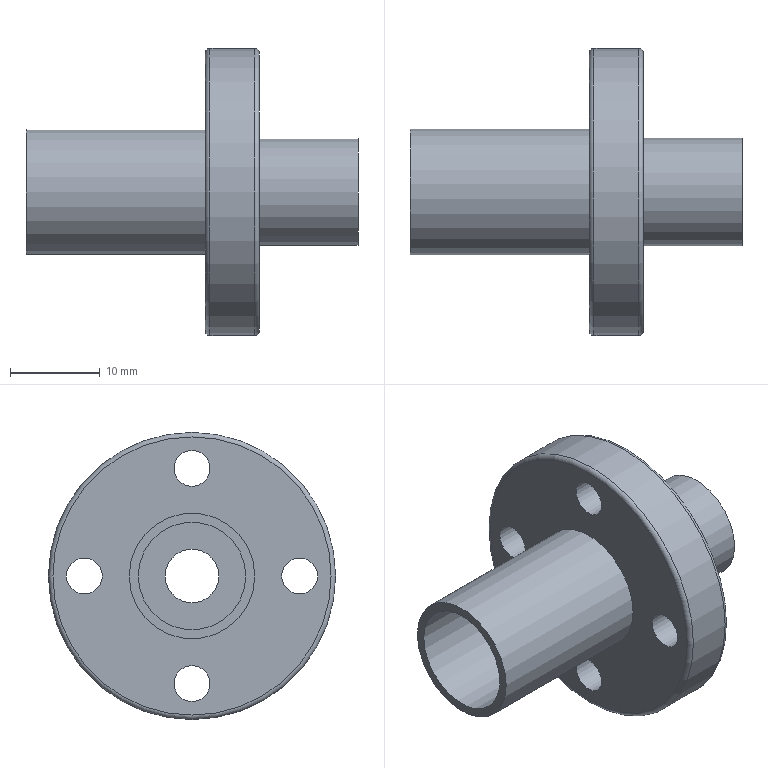Part | STEP file | 1-23.1 | 1 solid | 16 faces | box 37 x 32 x 32 mm | volume 6942 mm3 | cylinder 9 | plane 5 | torus 2 | commonest cylinder face diameters 4 x4 12 x2 6 x1 14 x1 32 x1
STEP:
#1=CARTESIAN_POINT('',(0.,0.,0.));
#2=DIRECTION('',(0.,0.,1.));
#3=DIRECTION('',(1.,0.,0.));
#4=AXIS2_PLACEMENT_3D('',#1,#2,#3);
#5=CARTESIAN_POINT('',(0.,2.,12.));
#6=VERTEX_POINT('',#5);
#7=CARTESIAN_POINT('',(6.,2.,12.));
#8=VERTEX_POINT('',#7);
#9=CARTESIAN_POINT('',(0.,2.,12.));
#10=DIRECTION('',(1.,0.,0.));
#11=VECTOR('',#10,1.);
#12=LINE('',#9,#11);
#13=CARTESIAN_POINT('',(0.,0.,12.));
#14=DIRECTION('',(1.,0.,0.));
#15=DIRECTION('',(0.,1.,0.));
#16=AXIS2_PLACEMENT_3D('',#13,#14,#15);
#17=CYLINDRICAL_SURFACE('',#16,2.);
#18=CARTESIAN_POINT('',(6.283,0.));
#19=DIRECTION('',(0.,1.));
#20=VECTOR('',#19,1.);
#21=LINE('',#18,#20);
#22=(GEOMETRIC_REPRESENTATION_CONTEXT(2)PARAMETRIC_REPRESENTATION_CONTEXT()REPRESENTATION_CONTEXT('',''));
#23=DEFINITIONAL_REPRESENTATION('',(#21),#22);
#24=PCURVE('',#17,#23);
#25=CARTESIAN_POINT('',(0.,0.));
#26=DIRECTION('',(0.,1.));
#27=VECTOR('',#26,1.);
#28=LINE('',#25,#27);
#29=(GEOMETRIC_REPRESENTATION_CONTEXT(2)PARAMETRIC_REPRESENTATION_CONTEXT()REPRESENTATION_CONTEXT('',''));
#30=DEFINITIONAL_REPRESENTATION('',(#28),#29);
#31=PCURVE('',#17,#30);
#32=SEAM_CURVE('',#12,(#24,#31),.PCURVE_S1.);
#33=EDGE_CURVE('',#6,#8,#32,.T.);
#34=ORIENTED_EDGE('',*,*,#33,.T.);
#35=CARTESIAN_POINT('',(6.,0.,12.));
#36=DIRECTION('',(-1.,0.,0.));
#37=DIRECTION('',(0.,1.,0.));
#38=AXIS2_PLACEMENT_3D('',#35,#36,#37);
#39=CIRCLE('',#38,2.);
#40=CARTESIAN_POINT('',(6.283,6.));
#41=DIRECTION('',(-1.,0.));
#42=VECTOR('',#41,1.);
#43=LINE('',#40,#42);
#44=(GEOMETRIC_REPRESENTATION_CONTEXT(2)PARAMETRIC_REPRESENTATION_CONTEXT()REPRESENTATION_CONTEXT('',''));
#45=DEFINITIONAL_REPRESENTATION('',(#43),#44);
#46=PCURVE('',#17,#45);
#47=CARTESIAN_POINT('',(6.,-4.287,0.));
#48=DIRECTION('',(1.,0.,0.));
#49=DIRECTION('',(0.,1.,0.));
#50=AXIS2_PLACEMENT_3D('',#47,#48,#49);
#51=PLANE('',#50);
#52=CARTESIAN_POINT('',(6.287,12.));
#53=CARTESIAN_POINT('',(6.287,8.536));
#54=CARTESIAN_POINT('',(3.287,10.268));
#55=CARTESIAN_POINT('',(0.2872,12.));
#56=CARTESIAN_POINT('',(3.287,13.732));
#57=CARTESIAN_POINT('',(6.287,15.464));
#58=CARTESIAN_POINT('',(6.287,12.));
#59=(BOUNDED_CURVE()B_SPLINE_CURVE(2,(#52,#53,#54,#55,#56,#57,#58),.UNSPECIFIED.,.T.,.F.)B_SPLINE_CURVE_WITH_KNOTS((1,2,2,2,2,1),(-2.094,0.,2.094,4.189,6.283,8.378),.UNSPECIFIED.)CURVE()GEOMETRIC_REPRESENTATION_ITEM()RATIONAL_B_SPLINE_CURVE((1.,0.5,1.,0.5,1.,0.5,1.))REPRESENTATION_ITEM(''));
#60=(GEOMETRIC_REPRESENTATION_CONTEXT(2)PARAMETRIC_REPRESENTATION_CONTEXT()REPRESENTATION_CONTEXT('',''));
#61=DEFINITIONAL_REPRESENTATION('',(#59),#60);
#62=PCURVE('',#51,#61);
#63=SURFACE_CURVE('',#39,(#46,#62),.PCURVE_S1.);
#64=EDGE_CURVE('',#8,#8,#63,.T.);
#65=ORIENTED_EDGE('',*,*,#64,.T.);
#66=ORIENTED_EDGE('',*,*,#33,.F.);
#67=CARTESIAN_POINT('',(0.,0.,12.));
#68=DIRECTION('',(-1.,0.,0.));
#69=DIRECTION('',(0.,1.,0.));
#70=AXIS2_PLACEMENT_3D('',#67,#68,#69);
#71=CIRCLE('',#70,2.);
#72=CARTESIAN_POINT('',(6.283,0.));
#73=DIRECTION('',(-1.,0.));
#74=VECTOR('',#73,1.);
#75=LINE('',#72,#74);
#76=(GEOMETRIC_REPRESENTATION_CONTEXT(2)PARAMETRIC_REPRESENTATION_CONTEXT()REPRESENTATION_CONTEXT('',''));
#77=DEFINITIONAL_REPRESENTATION('',(#75),#76);
#78=PCURVE('',#17,#77);
#79=CARTESIAN_POINT('',(0.,-4.287,0.));
#80=DIRECTION('',(1.,0.,0.));
#81=DIRECTION('',(0.,1.,0.));
#82=AXIS2_PLACEMENT_3D('',#79,#80,#81);
#83=PLANE('',#82);
#84=CARTESIAN_POINT('',(6.287,12.));
#85=CARTESIAN_POINT('',(6.287,8.536));
#86=CARTESIAN_POINT('',(3.287,10.268));
#87=CARTESIAN_POINT('',(0.2872,12.));
#88=CARTESIAN_POINT('',(3.287,13.732));
#89=CARTESIAN_POINT('',(6.287,15.464));
#90=CARTESIAN_POINT('',(6.287,12.));
#91=(BOUNDED_CURVE()B_SPLINE_CURVE(2,(#84,#85,#86,#87,#88,#89,#90),.UNSPECIFIED.,.T.,.F.)B_SPLINE_CURVE_WITH_KNOTS((1,2,2,2,2,1),(-2.094,0.,2.094,4.189,6.283,8.378),.UNSPECIFIED.)CURVE()GEOMETRIC_REPRESENTATION_ITEM()RATIONAL_B_SPLINE_CURVE((1.,0.5,1.,0.5,1.,0.5,1.))REPRESENTATION_ITEM(''));
#92=(GEOMETRIC_REPRESENTATION_CONTEXT(2)PARAMETRIC_REPRESENTATION_CONTEXT()REPRESENTATION_CONTEXT('',''));
#93=DEFINITIONAL_REPRESENTATION('',(#91),#92);
#94=PCURVE('',#83,#93);
#95=SURFACE_CURVE('',#71,(#78,#94),.PCURVE_S1.);
#96=EDGE_CURVE('',#6,#6,#95,.T.);
#97=ORIENTED_EDGE('',*,*,#96,.F.);
#98=EDGE_LOOP('',(#34,#65,#66,#97));
#99=FACE_BOUND('',#98,.F.);
#100=ADVANCED_FACE('',(#99),#17,.F.);
#101=CARTESIAN_POINT('',(0.,14.,0.));
#102=VERTEX_POINT('',#101);
#103=CARTESIAN_POINT('',(6.,14.,0.));
#104=VERTEX_POINT('',#103);
#105=CARTESIAN_POINT('',(0.,14.,0.));
#106=DIRECTION('',(1.,0.,0.));
#107=VECTOR('',#106,1.);
#108=LINE('',#105,#107);
#109=CARTESIAN_POINT('',(0.,12.,0.));
#110=DIRECTION('',(1.,0.,0.));
#111=DIRECTION('',(0.,1.,0.));
#112=AXIS2_PLACEMENT_3D('',#109,#110,#111);
#113=CYLINDRICAL_SURFACE('',#112,2.);
#114=CARTESIAN_POINT('',(6.283,0.));
#115=DIRECTION('',(0.,1.));
#116=VECTOR('',#115,1.);
#117=LINE('',#114,#116);
#118=(GEOMETRIC_REPRESENTATION_CONTEXT(2)PARAMETRIC_REPRESENTATION_CONTEXT()REPRESENTATION_CONTEXT('',''));
#119=DEFINITIONAL_REPRESENTATION('',(#117),#118);
#120=PCURVE('',#113,#119);
#121=CARTESIAN_POINT('',(0.,0.));
#122=DIRECTION('',(0.,1.));
#123=VECTOR('',#122,1.);
#124=LINE('',#121,#123);
#125=(GEOMETRIC_REPRESENTATION_CONTEXT(2)PARAMETRIC_REPRESENTATION_CONTEXT()REPRESENTATION_CONTEXT('',''));
#126=DEFINITIONAL_REPRESENTATION('',(#124),#125);
#127=PCURVE('',#113,#126);
#128=SEAM_CURVE('',#108,(#120,#127),.PCURVE_S1.);
#129=EDGE_CURVE('',#102,#104,#128,.T.);
#130=ORIENTED_EDGE('',*,*,#129,.T.);
#131=CARTESIAN_POINT('',(6.,12.,0.));
#132=DIRECTION('',(-1.,0.,0.));
#133=DIRECTION('',(0.,1.,0.));
#134=AXIS2_PLACEMENT_3D('',#131,#132,#133);
#135=CIRCLE('',#134,2.);
#136=CARTESIAN_POINT('',(6.283,6.));
#137=DIRECTION('',(-1.,0.));
#138=VECTOR('',#137,1.);
#139=LINE('',#136,#138);
#140=(GEOMETRIC_REPRESENTATION_CONTEXT(2)PARAMETRIC_REPRESENTATION_CONTEXT()REPRESENTATION_CONTEXT('',''));
#141=DEFINITIONAL_REPRESENTATION('',(#139),#140);
#142=PCURVE('',#113,#141);
#143=CARTESIAN_POINT('',(18.287,0.));
#144=CARTESIAN_POINT('',(18.287,-3.464));
#145=CARTESIAN_POINT('',(15.287,-1.732));
#146=CARTESIAN_POINT('',(12.287,0.));
#147=CARTESIAN_POINT('',(15.287,1.732));
#148=CARTESIAN_POINT('',(18.287,3.464));
#149=CARTESIAN_POINT('',(18.287,0.));
#150=(BOUNDED_CURVE()B_SPLINE_CURVE(2,(#143,#144,#145,#146,#147,#148,#149),.UNSPECIFIED.,.T.,.F.)B_SPLINE_CURVE_WITH_KNOTS((1,2,2,2,2,1),(-2.094,0.,2.094,4.189,6.283,8.378),.UNSPECIFIED.)CURVE()GEOMETRIC_REPRESENTATION_ITEM()RATIONAL_B_SPLINE_CURVE((1.,0.5,1.,0.5,1.,0.5,1.))REPRESENTATION_ITEM(''));
#151=(GEOMETRIC_REPRESENTATION_CONTEXT(2)PARAMETRIC_REPRESENTATION_CONTEXT()REPRESENTATION_CONTEXT('',''));
#152=DEFINITIONAL_REPRESENTATION('',(#150),#151);
#153=PCURVE('',#51,#152);
#154=SURFACE_CURVE('',#135,(#142,#153),.PCURVE_S1.);
#155=EDGE_CURVE('',#104,#104,#154,.T.);
#156=ORIENTED_EDGE('',*,*,#155,.T.);
#157=ORIENTED_EDGE('',*,*,#129,.F.);
#158=CARTESIAN_POINT('',(0.,12.,0.));
#159=DIRECTION('',(-1.,0.,0.));
#160=DIRECTION('',(0.,1.,0.));
#161=AXIS2_PLACEMENT_3D('',#158,#159,#160);
#162=CIRCLE('',#161,2.);
#163=CARTESIAN_POINT('',(6.283,0.));
#164=DIRECTION('',(-1.,0.));
#165=VECTOR('',#164,1.);
#166=LINE('',#163,#165);
#167=(GEOMETRIC_REPRESENTATION_CONTEXT(2)PARAMETRIC_REPRESENTATION_CONTEXT()REPRESENTATION_CONTEXT('',''));
#168=DEFINITIONAL_REPRESENTATION('',(#166),#167);
#169=PCURVE('',#113,#168);
#170=CARTESIAN_POINT('',(18.287,0.));
#171=CARTESIAN_POINT('',(18.287,-3.464));
#172=CARTESIAN_POINT('',(15.287,-1.732));
#173=CARTESIAN_POINT('',(12.287,0.));
#174=CARTESIAN_POINT('',(15.287,1.732));
#175=CARTESIAN_POINT('',(18.287,3.464));
#176=CARTESIAN_POINT('',(18.287,0.));
#177=(BOUNDED_CURVE()B_SPLINE_CURVE(2,(#170,#171,#172,#173,#174,#175,#176),.UNSPECIFIED.,.T.,.F.)B_SPLINE_CURVE_WITH_KNOTS((1,2,2,2,2,1),(-2.094,0.,2.094,4.189,6.283,8.378),.UNSPECIFIED.)CURVE()GEOMETRIC_REPRESENTATION_ITEM()RATIONAL_B_SPLINE_CURVE((1.,0.5,1.,0.5,1.,0.5,1.))REPRESENTATION_ITEM(''));
#178=(GEOMETRIC_REPRESENTATION_CONTEXT(2)PARAMETRIC_REPRESENTATION_CONTEXT()REPRESENTATION_CONTEXT('',''));
#179=DEFINITIONAL_REPRESENTATION('',(#177),#178);
#180=PCURVE('',#83,#179);
#181=SURFACE_CURVE('',#162,(#169,#180),.PCURVE_S1.);
#182=EDGE_CURVE('',#102,#102,#181,.T.);
#183=ORIENTED_EDGE('',*,*,#182,.F.);
#184=EDGE_LOOP('',(#130,#156,#157,#183));
#185=FACE_BOUND('',#184,.F.);
#186=ADVANCED_FACE('',(#185),#113,.F.);
#187=CARTESIAN_POINT('',(0.,2.,-12.));
#188=VERTEX_POINT('',#187);
#189=CARTESIAN_POINT('',(6.,2.,-12.));
#190=VERTEX_POINT('',#189);
#191=CARTESIAN_POINT('',(0.,2.,-12.));
#192=DIRECTION('',(1.,0.,0.));
#193=VECTOR('',#192,1.);
#194=LINE('',#191,#193);
#195=CARTESIAN_POINT('',(0.,0.,-12.));
#196=DIRECTION('',(1.,0.,0.));
#197=DIRECTION('',(0.,1.,0.));
#198=AXIS2_PLACEMENT_3D('',#195,#196,#197);
#199=CYLINDRICAL_SURFACE('',#198,2.);
#200=CARTESIAN_POINT('',(6.283,0.));
#201=DIRECTION('',(0.,1.));
#202=VECTOR('',#201,1.);
#203=LINE('',#200,#202);
#204=(GEOMETRIC_REPRESENTATION_CONTEXT(2)PARAMETRIC_REPRESENTATION_CONTEXT()REPRESENTATION_CONTEXT('',''));
#205=DEFINITIONAL_REPRESENTATION('',(#203),#204);
#206=PCURVE('',#199,#205);
#207=CARTESIAN_POINT('',(0.,0.));
#208=DIRECTION('',(0.,1.));
#209=VECTOR('',#208,1.);
#210=LINE('',#207,#209);
#211=(GEOMETRIC_REPRESENTATION_CONTEXT(2)PARAMETRIC_REPRESENTATION_CONTEXT()REPRESENTATION_CONTEXT('',''));
#212=DEFINITIONAL_REPRESENTATION('',(#210),#211);
#213=PCURVE('',#199,#212);
#214=SEAM_CURVE('',#194,(#206,#213),.PCURVE_S1.);
#215=EDGE_CURVE('',#188,#190,#214,.T.);
#216=ORIENTED_EDGE('',*,*,#215,.T.);
#217=CARTESIAN_POINT('',(6.,0.,-12.));
#218=DIRECTION('',(-1.,0.,0.));
#219=DIRECTION('',(0.,1.,0.));
#220=AXIS2_PLACEMENT_3D('',#217,#218,#219);
#221=CIRCLE('',#220,2.);
#222=CARTESIAN_POINT('',(6.283,6.));
#223=DIRECTION('',(-1.,0.));
#224=VECTOR('',#223,1.);
#225=LINE('',#222,#224);
#226=(GEOMETRIC_REPRESENTATION_CONTEXT(2)PARAMETRIC_REPRESENTATION_CONTEXT()REPRESENTATION_CONTEXT('',''));
#227=DEFINITIONAL_REPRESENTATION('',(#225),#226);
#228=PCURVE('',#199,#227);
#229=CARTESIAN_POINT('',(6.287,-12.));
#230=CARTESIAN_POINT('',(6.287,-15.464));
#231=CARTESIAN_POINT('',(3.287,-13.732));
#232=CARTESIAN_POINT('',(0.2872,-12.));
#233=CARTESIAN_POINT('',(3.287,-10.268));
#234=CARTESIAN_POINT('',(6.287,-8.536));
#235=CARTESIAN_POINT('',(6.287,-12.));
#236=(BOUNDED_CURVE()B_SPLINE_CURVE(2,(#229,#230,#231,#232,#233,#234,#235),.UNSPECIFIED.,.T.,.F.)B_SPLINE_CURVE_WITH_KNOTS((1,2,2,2,2,1),(-2.094,0.,2.094,4.189,6.283,8.378),.UNSPECIFIED.)CURVE()GEOMETRIC_REPRESENTATION_ITEM()RATIONAL_B_SPLINE_CURVE((1.,0.5,1.,0.5,1.,0.5,1.))REPRESENTATION_ITEM(''));
#237=(GEOMETRIC_REPRESENTATION_CONTEXT(2)PARAMETRIC_REPRESENTATION_CONTEXT()REPRESENTATION_CONTEXT('',''));
#238=DEFINITIONAL_REPRESENTATION('',(#236),#237);
#239=PCURVE('',#51,#238);
#240=SURFACE_CURVE('',#221,(#228,#239),.PCURVE_S1.);
#241=EDGE_CURVE('',#190,#190,#240,.T.);
#242=ORIENTED_EDGE('',*,*,#241,.T.);
#243=ORIENTED_EDGE('',*,*,#215,.F.);
#244=CARTESIAN_POINT('',(0.,0.,-12.));
#245=DIRECTION('',(-1.,0.,0.));
#246=DIRECTION('',(0.,1.,0.));
#247=AXIS2_PLACEMENT_3D('',#244,#245,#246);
#248=CIRCLE('',#247,2.);
#249=CARTESIAN_POINT('',(6.283,0.));
#250=DIRECTION('',(-1.,0.));
#251=VECTOR('',#250,1.);
#252=LINE('',#249,#251);
#253=(GEOMETRIC_REPRESENTATION_CONTEXT(2)PARAMETRIC_REPRESENTATION_CONTEXT()REPRESENTATION_CONTEXT('',''));
#254=DEFINITIONAL_REPRESENTATION('',(#252),#253);
#255=PCURVE('',#199,#254);
#256=CARTESIAN_POINT('',(6.287,-12.));
#257=CARTESIAN_POINT('',(6.287,-15.464));
#258=CARTESIAN_POINT('',(3.287,-13.732));
#259=CARTESIAN_POINT('',(0.2872,-12.));
#260=CARTESIAN_POINT('',(3.287,-10.268));
#261=CARTESIAN_POINT('',(6.287,-8.536));
#262=CARTESIAN_POINT('',(6.287,-12.));
#263=(BOUNDED_CURVE()B_SPLINE_CURVE(2,(#256,#257,#258,#259,#260,#261,#262),.UNSPECIFIED.,.T.,.F.)B_SPLINE_CURVE_WITH_KNOTS((1,2,2,2,2,1),(-2.094,0.,2.094,4.189,6.283,8.378),.UNSPECIFIED.)CURVE()GEOMETRIC_REPRESENTATION_ITEM()RATIONAL_B_SPLINE_CURVE((1.,0.5,1.,0.5,1.,0.5,1.))REPRESENTATION_ITEM(''));
#264=(GEOMETRIC_REPRESENTATION_CONTEXT(2)PARAMETRIC_REPRESENTATION_CONTEXT()REPRESENTATION_CONTEXT('',''));
#265=DEFINITIONAL_REPRESENTATION('',(#263),#264);
#266=PCURVE('',#83,#265);
#267=SURFACE_CURVE('',#248,(#255,#266),.PCURVE_S1.);
#268=EDGE_CURVE('',#188,#188,#267,.T.);
#269=ORIENTED_EDGE('',*,*,#268,.F.);
#270=EDGE_LOOP('',(#216,#242,#243,#269));
#271=FACE_BOUND('',#270,.F.);
#272=ADVANCED_FACE('',(#271),#199,.F.);
#273=CARTESIAN_POINT('',(0.,-10.,0.));
#274=VERTEX_POINT('',#273);
#275=CARTESIAN_POINT('',(6.,-10.,0.));
#276=VERTEX_POINT('',#275);
#277=CARTESIAN_POINT('',(0.,-10.,0.));
#278=DIRECTION('',(1.,0.,0.));
#279=VECTOR('',#278,1.);
#280=LINE('',#277,#279);
#281=CARTESIAN_POINT('',(0.,-12.,0.));
#282=DIRECTION('',(1.,0.,0.));
#283=DIRECTION('',(0.,1.,0.));
#284=AXIS2_PLACEMENT_3D('',#281,#282,#283);
#285=CYLINDRICAL_SURFACE('',#284,2.);
#286=CARTESIAN_POINT('',(6.283,0.));
#287=DIRECTION('',(0.,1.));
#288=VECTOR('',#287,1.);
#289=LINE('',#286,#288);
#290=(GEOMETRIC_REPRESENTATION_CONTEXT(2)PARAMETRIC_REPRESENTATION_CONTEXT()REPRESENTATION_CONTEXT('',''));
#291=DEFINITIONAL_REPRESENTATION('',(#289),#290);
#292=PCURVE('',#285,#291);
#293=CARTESIAN_POINT('',(0.,0.));
#294=DIRECTION('',(0.,1.));
#295=VECTOR('',#294,1.);
#296=LINE('',#293,#295);
#297=(GEOMETRIC_REPRESENTATION_CONTEXT(2)PARAMETRIC_REPRESENTATION_CONTEXT()REPRESENTATION_CONTEXT('',''));
#298=DEFINITIONAL_REPRESENTATION('',(#296),#297);
#299=PCURVE('',#285,#298);
#300=SEAM_CURVE('',#280,(#292,#299),.PCURVE_S1.);
#301=EDGE_CURVE('',#274,#276,#300,.T.);
#302=ORIENTED_EDGE('',*,*,#301,.T.);
#303=CARTESIAN_POINT('',(6.,-12.,0.));
#304=DIRECTION('',(-1.,0.,0.));
#305=DIRECTION('',(0.,1.,0.));
#306=AXIS2_PLACEMENT_3D('',#303,#304,#305);
#307=CIRCLE('',#306,2.);
#308=CARTESIAN_POINT('',(6.283,6.));
#309=DIRECTION('',(-1.,0.));
#310=VECTOR('',#309,1.);
#311=LINE('',#308,#310);
#312=(GEOMETRIC_REPRESENTATION_CONTEXT(2)PARAMETRIC_REPRESENTATION_CONTEXT()REPRESENTATION_CONTEXT('',''));
#313=DEFINITIONAL_REPRESENTATION('',(#311),#312);
#314=PCURVE('',#285,#313);
#315=CARTESIAN_POINT('',(-5.713,0.));
#316=CARTESIAN_POINT('',(-5.713,-3.464));
#317=CARTESIAN_POINT('',(-8.713,-1.732));
#318=CARTESIAN_POINT('',(-11.713,0.));
#319=CARTESIAN_POINT('',(-8.713,1.732));
#320=CARTESIAN_POINT('',(-5.713,3.464));
#321=CARTESIAN_POINT('',(-5.713,0.));
#322=(BOUNDED_CURVE()B_SPLINE_CURVE(2,(#315,#316,#317,#318,#319,#320,#321),.UNSPECIFIED.,.T.,.F.)B_SPLINE_CURVE_WITH_KNOTS((1,2,2,2,2,1),(-2.094,0.,2.094,4.189,6.283,8.378),.UNSPECIFIED.)CURVE()GEOMETRIC_REPRESENTATION_ITEM()RATIONAL_B_SPLINE_CURVE((1.,0.5,1.,0.5,1.,0.5,1.))REPRESENTATION_ITEM(''));
#323=(GEOMETRIC_REPRESENTATION_CONTEXT(2)PARAMETRIC_REPRESENTATION_CONTEXT()REPRESENTATION_CONTEXT('',''));
#324=DEFINITIONAL_REPRESENTATION('',(#322),#323);
#325=PCURVE('',#51,#324);
#326=SURFACE_CURVE('',#307,(#314,#325),.PCURVE_S1.);
#327=EDGE_CURVE('',#276,#276,#326,.T.);
#328=ORIENTED_EDGE('',*,*,#327,.T.);
#329=ORIENTED_EDGE('',*,*,#301,.F.);
#330=CARTESIAN_POINT('',(0.,-12.,0.));
#331=DIRECTION('',(-1.,0.,0.));
#332=DIRECTION('',(0.,1.,0.));
#333=AXIS2_PLACEMENT_3D('',#330,#331,#332);
#334=CIRCLE('',#333,2.);
#335=CARTESIAN_POINT('',(6.283,0.));
#336=DIRECTION('',(-1.,0.));
#337=VECTOR('',#336,1.);
#338=LINE('',#335,#337);
#339=(GEOMETRIC_REPRESENTATION_CONTEXT(2)PARAMETRIC_REPRESENTATION_CONTEXT()REPRESENTATION_CONTEXT('',''));
#340=DEFINITIONAL_REPRESENTATION('',(#338),#339);
#341=PCURVE('',#285,#340);
#342=CARTESIAN_POINT('',(-5.713,0.));
#343=CARTESIAN_POINT('',(-5.713,-3.464));
#344=CARTESIAN_POINT('',(-8.713,-1.732));
#345=CARTESIAN_POINT('',(-11.713,0.));
#346=CARTESIAN_POINT('',(-8.713,1.732));
#347=CARTESIAN_POINT('',(-5.713,3.464));
#348=CARTESIAN_POINT('',(-5.713,0.));
#349=(BOUNDED_CURVE()B_SPLINE_CURVE(2,(#342,#343,#344,#345,#346,#347,#348),.UNSPECIFIED.,.T.,.F.)B_SPLINE_CURVE_WITH_KNOTS((1,2,2,2,2,1),(-2.094,0.,2.094,4.189,6.283,8.378),.UNSPECIFIED.)CURVE()GEOMETRIC_REPRESENTATION_ITEM()RATIONAL_B_SPLINE_CURVE((1.,0.5,1.,0.5,1.,0.5,1.))REPRESENTATION_ITEM(''));
#350=(GEOMETRIC_REPRESENTATION_CONTEXT(2)PARAMETRIC_REPRESENTATION_CONTEXT()REPRESENTATION_CONTEXT('',''));
#351=DEFINITIONAL_REPRESENTATION('',(#349),#350);
#352=PCURVE('',#83,#351);
#353=SURFACE_CURVE('',#334,(#341,#352),.PCURVE_S1.);
#354=EDGE_CURVE('',#274,#274,#353,.T.);
#355=ORIENTED_EDGE('',*,*,#354,.F.);
#356=EDGE_LOOP('',(#302,#328,#329,#355));
#357=FACE_BOUND('',#356,.F.);
#358=ADVANCED_FACE('',(#357),#285,.F.);
#359=CARTESIAN_POINT('',(6.,6.,0.));
#360=VERTEX_POINT('',#359);
#361=CARTESIAN_POINT('',(6.,0.,0.));
#362=DIRECTION('',(1.,0.,0.));
#363=DIRECTION('',(0.,1.,0.));
#364=AXIS2_PLACEMENT_3D('',#361,#362,#363);
#365=CIRCLE('',#364,6.);
#366=CARTESIAN_POINT('',(6.,0.,0.));
#367=DIRECTION('',(1.,0.,0.));
#368=DIRECTION('',(0.,1.,0.));
#369=AXIS2_PLACEMENT_3D('',#366,#367,#368);
#370=CYLINDRICAL_SURFACE('',#369,6.);
#371=CARTESIAN_POINT('',(0.,0.));
#372=DIRECTION('',(1.,0.));
#373=VECTOR('',#372,1.);
#374=LINE('',#371,#373);
#375=(GEOMETRIC_REPRESENTATION_CONTEXT(2)PARAMETRIC_REPRESENTATION_CONTEXT()REPRESENTATION_CONTEXT('',''));
#376=DEFINITIONAL_REPRESENTATION('',(#374),#375);
#377=PCURVE('',#370,#376);
#378=CARTESIAN_POINT('',(4.287,0.));
#379=DIRECTION('',(1.,0.));
#380=AXIS2_PLACEMENT_2D('',#378,#379);
#381=CIRCLE('',#380,6.);
#382=(GEOMETRIC_REPRESENTATION_CONTEXT(2)PARAMETRIC_REPRESENTATION_CONTEXT()REPRESENTATION_CONTEXT('',''));
#383=DEFINITIONAL_REPRESENTATION('',(#381),#382);
#384=PCURVE('',#51,#383);
#385=SURFACE_CURVE('',#365,(#377,#384),.PCURVE_S1.);
#386=EDGE_CURVE('',#360,#360,#385,.T.);
#387=ORIENTED_EDGE('',*,*,#386,.T.);
#388=CARTESIAN_POINT('',(17.,6.,0.));
#389=VERTEX_POINT('',#388);
#390=CARTESIAN_POINT('',(6.,6.,0.));
#391=DIRECTION('',(1.,0.,0.));
#392=VECTOR('',#391,1.);
#393=LINE('',#390,#392);
#394=CARTESIAN_POINT('',(6.283,0.));
#395=DIRECTION('',(0.,1.));
#396=VECTOR('',#395,1.);
#397=LINE('',#394,#396);
#398=(GEOMETRIC_REPRESENTATION_CONTEXT(2)PARAMETRIC_REPRESENTATION_CONTEXT()REPRESENTATION_CONTEXT('',''));
#399=DEFINITIONAL_REPRESENTATION('',(#397),#398);
#400=PCURVE('',#370,#399);
#401=CARTESIAN_POINT('',(0.,0.));
#402=DIRECTION('',(0.,1.));
#403=VECTOR('',#402,1.);
#404=LINE('',#401,#403);
#405=(GEOMETRIC_REPRESENTATION_CONTEXT(2)PARAMETRIC_REPRESENTATION_CONTEXT()REPRESENTATION_CONTEXT('',''));
#406=DEFINITIONAL_REPRESENTATION('',(#404),#405);
#407=PCURVE('',#370,#406);
#408=SEAM_CURVE('',#393,(#400,#407),.PCURVE_S1.);
#409=EDGE_CURVE('',#360,#389,#408,.T.);
#410=ORIENTED_EDGE('',*,*,#409,.T.);
#411=CARTESIAN_POINT('',(17.,0.,0.));
#412=DIRECTION('',(1.,0.,0.));
#413=DIRECTION('',(0.,1.,0.));
#414=AXIS2_PLACEMENT_3D('',#411,#412,#413);
#415=CIRCLE('',#414,6.);
#416=CARTESIAN_POINT('',(0.,11.));
#417=DIRECTION('',(1.,0.));
#418=VECTOR('',#417,1.);
#419=LINE('',#416,#418);
#420=(GEOMETRIC_REPRESENTATION_CONTEXT(2)PARAMETRIC_REPRESENTATION_CONTEXT()REPRESENTATION_CONTEXT('',''));
#421=DEFINITIONAL_REPRESENTATION('',(#419),#420);
#422=PCURVE('',#370,#421);
#423=CARTESIAN_POINT('',(17.,-1.608,0.));
#424=DIRECTION('',(1.,0.,0.));
#425=DIRECTION('',(0.,1.,0.));
#426=AXIS2_PLACEMENT_3D('',#423,#424,#425);
#427=PLANE('',#426);
#428=CARTESIAN_POINT('',(1.608,0.));
#429=DIRECTION('',(1.,0.));
#430=AXIS2_PLACEMENT_2D('',#428,#429);
#431=CIRCLE('',#430,6.);
#432=(GEOMETRIC_REPRESENTATION_CONTEXT(2)PARAMETRIC_REPRESENTATION_CONTEXT()REPRESENTATION_CONTEXT('',''));
#433=DEFINITIONAL_REPRESENTATION('',(#431),#432);
#434=PCURVE('',#427,#433);
#435=SURFACE_CURVE('',#415,(#422,#434),.PCURVE_S1.);
#436=EDGE_CURVE('',#389,#389,#435,.T.);
#437=ORIENTED_EDGE('',*,*,#436,.F.);
#438=ORIENTED_EDGE('',*,*,#409,.F.);
#439=EDGE_LOOP('',(#387,#410,#437,#438));
#440=FACE_BOUND('',#439,.T.);
#441=ADVANCED_FACE('',(#440),#370,.T.);
#442=CARTESIAN_POINT('',(0.,-7.,0.));
#443=VERTEX_POINT('',#442);
#444=CARTESIAN_POINT('',(0.,0.,0.));
#445=DIRECTION('',(-1.,0.,0.));
#446=DIRECTION('',(0.,-1.,0.));
#447=AXIS2_PLACEMENT_3D('',#444,#445,#446);
#448=CIRCLE('',#447,7.);
#449=CARTESIAN_POINT('',(0.,0.,0.));
#450=DIRECTION('',(-1.,0.,0.));
#451=DIRECTION('',(0.,-1.,0.));
#452=AXIS2_PLACEMENT_3D('',#449,#450,#451);
#453=CYLINDRICAL_SURFACE('',#452,7.);
#454=CARTESIAN_POINT('',(0.,0.));
#455=DIRECTION('',(1.,0.));
#456=VECTOR('',#455,1.);
#457=LINE('',#454,#456);
#458=(GEOMETRIC_REPRESENTATION_CONTEXT(2)PARAMETRIC_REPRESENTATION_CONTEXT()REPRESENTATION_CONTEXT('',''));
#459=DEFINITIONAL_REPRESENTATION('',(#457),#458);
#460=PCURVE('',#453,#459);
#461=CARTESIAN_POINT('',(-2.713,0.));
#462=CARTESIAN_POINT('',(-2.713,12.124));
#463=CARTESIAN_POINT('',(7.787,6.062));
#464=CARTESIAN_POINT('',(18.287,0.));
#465=CARTESIAN_POINT('',(7.787,-6.062));
#466=CARTESIAN_POINT('',(-2.713,-12.124));
#467=CARTESIAN_POINT('',(-2.713,0.));
#468=(BOUNDED_CURVE()B_SPLINE_CURVE(2,(#461,#462,#463,#464,#465,#466,#467),.UNSPECIFIED.,.T.,.F.)B_SPLINE_CURVE_WITH_KNOTS((1,2,2,2,2,1),(-2.094,0.,2.094,4.189,6.283,8.378),.UNSPECIFIED.)CURVE()GEOMETRIC_REPRESENTATION_ITEM()RATIONAL_B_SPLINE_CURVE((1.,0.5,1.,0.5,1.,0.5,1.))REPRESENTATION_ITEM(''));
#469=(GEOMETRIC_REPRESENTATION_CONTEXT(2)PARAMETRIC_REPRESENTATION_CONTEXT()REPRESENTATION_CONTEXT('',''));
#470=DEFINITIONAL_REPRESENTATION('',(#468),#469);
#471=PCURVE('',#83,#470);
#472=SURFACE_CURVE('',#448,(#460,#471),.PCURVE_S1.);
#473=EDGE_CURVE('',#443,#443,#472,.T.);
#474=ORIENTED_EDGE('',*,*,#473,.T.);
#475=CARTESIAN_POINT('',(-20.,-7.,0.));
#476=VERTEX_POINT('',#475);
#477=CARTESIAN_POINT('',(0.,-7.,0.));
#478=DIRECTION('',(-1.,0.,0.));
#479=VECTOR('',#478,1.);
#480=LINE('',#477,#479);
#481=CARTESIAN_POINT('',(6.283,0.));
#482=DIRECTION('',(0.,1.));
#483=VECTOR('',#482,1.);
#484=LINE('',#481,#483);
#485=(GEOMETRIC_REPRESENTATION_CONTEXT(2)PARAMETRIC_REPRESENTATION_CONTEXT()REPRESENTATION_CONTEXT('',''));
#486=DEFINITIONAL_REPRESENTATION('',(#484),#485);
#487=PCURVE('',#453,#486);
#488=CARTESIAN_POINT('',(0.,0.));
#489=DIRECTION('',(0.,1.));
#490=VECTOR('',#489,1.);
#491=LINE('',#488,#490);
#492=(GEOMETRIC_REPRESENTATION_CONTEXT(2)PARAMETRIC_REPRESENTATION_CONTEXT()REPRESENTATION_CONTEXT('',''));
#493=DEFINITIONAL_REPRESENTATION('',(#491),#492);
#494=PCURVE('',#453,#493);
#495=SEAM_CURVE('',#480,(#487,#494),.PCURVE_S1.);
#496=EDGE_CURVE('',#443,#476,#495,.T.);
#497=ORIENTED_EDGE('',*,*,#496,.T.);
#498=CARTESIAN_POINT('',(-20.,0.,0.));
#499=DIRECTION('',(-1.,0.,0.));
#500=DIRECTION('',(0.,-1.,0.));
#501=AXIS2_PLACEMENT_3D('',#498,#499,#500);
#502=CIRCLE('',#501,7.);
#503=CARTESIAN_POINT('',(0.,20.));
#504=DIRECTION('',(1.,0.));
#505=VECTOR('',#504,1.);
#506=LINE('',#503,#505);
#507=(GEOMETRIC_REPRESENTATION_CONTEXT(2)PARAMETRIC_REPRESENTATION_CONTEXT()REPRESENTATION_CONTEXT('',''));
#508=DEFINITIONAL_REPRESENTATION('',(#506),#507);
#509=PCURVE('',#453,#508);
#510=CARTESIAN_POINT('',(-20.,1.876,0.));
#511=DIRECTION('',(-1.,0.,0.));
#512=DIRECTION('',(0.,-1.,0.));
#513=AXIS2_PLACEMENT_3D('',#510,#511,#512);
#514=PLANE('',#513);
#515=CARTESIAN_POINT('',(1.876,0.));
#516=DIRECTION('',(1.,0.));
#517=AXIS2_PLACEMENT_2D('',#515,#516);
#518=CIRCLE('',#517,7.);
#519=(GEOMETRIC_REPRESENTATION_CONTEXT(2)PARAMETRIC_REPRESENTATION_CONTEXT()REPRESENTATION_CONTEXT('',''));
#520=DEFINITIONAL_REPRESENTATION('',(#518),#519);
#521=PCURVE('',#514,#520);
#522=SURFACE_CURVE('',#502,(#509,#521),.PCURVE_S1.);
#523=EDGE_CURVE('',#476,#476,#522,.T.);
#524=ORIENTED_EDGE('',*,*,#523,.F.);
#525=ORIENTED_EDGE('',*,*,#496,.F.);
#526=EDGE_LOOP('',(#474,#497,#524,#525));
#527=FACE_BOUND('',#526,.T.);
#528=ADVANCED_FACE('',(#527),#453,.T.);
#529=ORIENTED_EDGE('',*,*,#523,.T.);
#530=EDGE_LOOP('',(#529));
#531=FACE_BOUND('',#530,.T.);
#532=CARTESIAN_POINT('',(-20.,-6.,0.));
#533=VERTEX_POINT('',#532);
#534=CARTESIAN_POINT('',(-20.,0.,0.));
#535=DIRECTION('',(-1.,0.,0.));
#536=DIRECTION('',(0.,-1.,0.));
#537=AXIS2_PLACEMENT_3D('',#534,#535,#536);
#538=CIRCLE('',#537,6.);
#539=CARTESIAN_POINT('',(1.876,0.));
#540=DIRECTION('',(1.,0.));
#541=AXIS2_PLACEMENT_2D('',#539,#540);
#542=CIRCLE('',#541,6.);
#543=(GEOMETRIC_REPRESENTATION_CONTEXT(2)PARAMETRIC_REPRESENTATION_CONTEXT()REPRESENTATION_CONTEXT('',''));
#544=DEFINITIONAL_REPRESENTATION('',(#542),#543);
#545=PCURVE('',#514,#544);
#546=CARTESIAN_POINT('',(-20.,0.,0.));
#547=DIRECTION('',(1.,0.,0.));
#548=DIRECTION('',(0.,-1.,0.));
#549=AXIS2_PLACEMENT_3D('',#546,#547,#548);
#550=CYLINDRICAL_SURFACE('',#549,6.);
#551=CARTESIAN_POINT('',(6.283,0.));
#552=DIRECTION('',(-1.,0.));
#553=VECTOR('',#552,1.);
#554=LINE('',#551,#553);
#555=(GEOMETRIC_REPRESENTATION_CONTEXT(2)PARAMETRIC_REPRESENTATION_CONTEXT()REPRESENTATION_CONTEXT('',''));
#556=DEFINITIONAL_REPRESENTATION('',(#554),#555);
#557=PCURVE('',#550,#556);
#558=SURFACE_CURVE('',#538,(#545,#557),.PCURVE_S1.);
#559=EDGE_CURVE('',#533,#533,#558,.T.);
#560=ORIENTED_EDGE('',*,*,#559,.F.);
#561=EDGE_LOOP('',(#560));
#562=FACE_BOUND('',#561,.T.);
#563=ADVANCED_FACE('',(#531,#562),#514,.T.);
#564=CARTESIAN_POINT('',(-10.,-6.,0.));
#565=VERTEX_POINT('',#564);
#566=CARTESIAN_POINT('',(-20.,-6.,0.));
#567=DIRECTION('',(1.,0.,0.));
#568=VECTOR('',#567,1.);
#569=LINE('',#566,#568);
#570=CARTESIAN_POINT('',(6.283,0.));
#571=DIRECTION('',(0.,1.));
#572=VECTOR('',#571,1.);
#573=LINE('',#570,#572);
#574=(GEOMETRIC_REPRESENTATION_CONTEXT(2)PARAMETRIC_REPRESENTATION_CONTEXT()REPRESENTATION_CONTEXT('',''));
#575=DEFINITIONAL_REPRESENTATION('',(#573),#574);
#576=PCURVE('',#550,#575);
#577=CARTESIAN_POINT('',(0.,0.));
#578=DIRECTION('',(0.,1.));
#579=VECTOR('',#578,1.);
#580=LINE('',#577,#579);
#581=(GEOMETRIC_REPRESENTATION_CONTEXT(2)PARAMETRIC_REPRESENTATION_CONTEXT()REPRESENTATION_CONTEXT('',''));
#582=DEFINITIONAL_REPRESENTATION('',(#580),#581);
#583=PCURVE('',#550,#582);
#584=SEAM_CURVE('',#569,(#576,#583),.PCURVE_S1.);
#585=EDGE_CURVE('',#533,#565,#584,.T.);
#586=ORIENTED_EDGE('',*,*,#585,.T.);
#587=CARTESIAN_POINT('',(-10.,0.,0.));
#588=DIRECTION('',(-1.,0.,0.));
#589=DIRECTION('',(0.,-1.,0.));
#590=AXIS2_PLACEMENT_3D('',#587,#588,#589);
#591=CIRCLE('',#590,6.);
#592=CARTESIAN_POINT('',(6.283,10.));
#593=DIRECTION('',(-1.,0.));
#594=VECTOR('',#593,1.);
#595=LINE('',#592,#594);
#596=(GEOMETRIC_REPRESENTATION_CONTEXT(2)PARAMETRIC_REPRESENTATION_CONTEXT()REPRESENTATION_CONTEXT('',''));
#597=DEFINITIONAL_REPRESENTATION('',(#595),#596);
#598=PCURVE('',#550,#597);
#599=CARTESIAN_POINT('',(-10.,1.608,0.));
#600=DIRECTION('',(-1.,0.,0.));
#601=DIRECTION('',(0.,-1.,0.));
#602=AXIS2_PLACEMENT_3D('',#599,#600,#601);
#603=PLANE('',#602);
#604=CARTESIAN_POINT('',(1.608,0.));
#605=DIRECTION('',(1.,0.));
#606=AXIS2_PLACEMENT_2D('',#604,#605);
#607=CIRCLE('',#606,6.);
#608=(GEOMETRIC_REPRESENTATION_CONTEXT(2)PARAMETRIC_REPRESENTATION_CONTEXT()REPRESENTATION_CONTEXT('',''));
#609=DEFINITIONAL_REPRESENTATION('',(#607),#608);
#610=PCURVE('',#603,#609);
#611=SURFACE_CURVE('',#591,(#598,#610),.PCURVE_S1.);
#612=EDGE_CURVE('',#565,#565,#611,.T.);
#613=ORIENTED_EDGE('',*,*,#612,.T.);
#614=ORIENTED_EDGE('',*,*,#585,.F.);
#615=ORIENTED_EDGE('',*,*,#559,.F.);
#616=EDGE_LOOP('',(#586,#613,#614,#615));
#617=FACE_BOUND('',#616,.F.);
#618=ADVANCED_FACE('',(#617),#550,.F.);
#619=ORIENTED_EDGE('',*,*,#436,.T.);
#620=EDGE_LOOP('',(#619));
#621=FACE_BOUND('',#620,.T.);
#622=CARTESIAN_POINT('',(17.,3.,0.));
#623=VERTEX_POINT('',#622);
#624=CARTESIAN_POINT('',(17.,0.,0.));
#625=DIRECTION('',(1.,0.,0.));
#626=DIRECTION('',(0.,1.,0.));
#627=AXIS2_PLACEMENT_3D('',#624,#625,#626);
#628=CIRCLE('',#627,3.);
#629=CARTESIAN_POINT('',(1.608,0.));
#630=DIRECTION('',(1.,0.));
#631=AXIS2_PLACEMENT_2D('',#629,#630);
#632=CIRCLE('',#631,3.);
#633=(GEOMETRIC_REPRESENTATION_CONTEXT(2)PARAMETRIC_REPRESENTATION_CONTEXT()REPRESENTATION_CONTEXT('',''));
#634=DEFINITIONAL_REPRESENTATION('',(#632),#633);
#635=PCURVE('',#427,#634);
#636=CARTESIAN_POINT('',(17.,0.,0.));
#637=DIRECTION('',(-1.,0.,0.));
#638=DIRECTION('',(0.,1.,0.));
#639=AXIS2_PLACEMENT_3D('',#636,#637,#638);
#640=CYLINDRICAL_SURFACE('',#639,3.);
#641=CARTESIAN_POINT('',(6.283,0.));
#642=DIRECTION('',(-1.,0.));
#643=VECTOR('',#642,1.);
#644=LINE('',#641,#643);
#645=(GEOMETRIC_REPRESENTATION_CONTEXT(2)PARAMETRIC_REPRESENTATION_CONTEXT()REPRESENTATION_CONTEXT('',''));
#646=DEFINITIONAL_REPRESENTATION('',(#644),#645);
#647=PCURVE('',#640,#646);
#648=SURFACE_CURVE('',#628,(#635,#647),.PCURVE_S1.);
#649=EDGE_CURVE('',#623,#623,#648,.T.);
#650=ORIENTED_EDGE('',*,*,#649,.F.);
#651=EDGE_LOOP('',(#650));
#652=FACE_BOUND('',#651,.T.);
#653=ADVANCED_FACE('',(#621,#652),#427,.T.);
#654=ORIENTED_EDGE('',*,*,#612,.T.);
#655=EDGE_LOOP('',(#654));
#656=FACE_BOUND('',#655,.T.);
#657=CARTESIAN_POINT('',(-10.,3.,0.));
#658=VERTEX_POINT('',#657);
#659=CARTESIAN_POINT('',(-10.,0.,0.));
#660=DIRECTION('',(-1.,0.,0.));
#661=DIRECTION('',(0.,1.,0.));
#662=AXIS2_PLACEMENT_3D('',#659,#660,#661);
#663=CIRCLE('',#662,3.);
#664=CARTESIAN_POINT('',(1.608,0.));
#665=DIRECTION('',(-1.,0.));
#666=AXIS2_PLACEMENT_2D('',#664,#665);
#667=CIRCLE('',#666,3.);
#668=(GEOMETRIC_REPRESENTATION_CONTEXT(2)PARAMETRIC_REPRESENTATION_CONTEXT()REPRESENTATION_CONTEXT('',''));
#669=DEFINITIONAL_REPRESENTATION('',(#667),#668);
#670=PCURVE('',#603,#669);
#671=CARTESIAN_POINT('',(0.,27.));
#672=DIRECTION('',(1.,0.));
#673=VECTOR('',#672,1.);
#674=LINE('',#671,#673);
#675=(GEOMETRIC_REPRESENTATION_CONTEXT(2)PARAMETRIC_REPRESENTATION_CONTEXT()REPRESENTATION_CONTEXT('',''));
#676=DEFINITIONAL_REPRESENTATION('',(#674),#675);
#677=PCURVE('',#640,#676);
#678=SURFACE_CURVE('',#663,(#670,#677),.PCURVE_S1.);
#679=EDGE_CURVE('',#658,#658,#678,.T.);
#680=ORIENTED_EDGE('',*,*,#679,.F.);
#681=EDGE_LOOP('',(#680));
#682=FACE_BOUND('',#681,.T.);
#683=ADVANCED_FACE('',(#656,#682),#603,.T.);
#684=CARTESIAN_POINT('',(17.,3.,0.));
#685=DIRECTION('',(-1.,0.,0.));
#686=VECTOR('',#685,1.);
#687=LINE('',#684,#686);
#688=CARTESIAN_POINT('',(6.283,0.));
#689=DIRECTION('',(0.,1.));
#690=VECTOR('',#689,1.);
#691=LINE('',#688,#690);
#692=(GEOMETRIC_REPRESENTATION_CONTEXT(2)PARAMETRIC_REPRESENTATION_CONTEXT()REPRESENTATION_CONTEXT('',''));
#693=DEFINITIONAL_REPRESENTATION('',(#691),#692);
#694=PCURVE('',#640,#693);
#695=CARTESIAN_POINT('',(0.,0.));
#696=DIRECTION('',(0.,1.));
#697=VECTOR('',#696,1.);
#698=LINE('',#695,#697);
#699=(GEOMETRIC_REPRESENTATION_CONTEXT(2)PARAMETRIC_REPRESENTATION_CONTEXT()REPRESENTATION_CONTEXT('',''));
#700=DEFINITIONAL_REPRESENTATION('',(#698),#699);
#701=PCURVE('',#640,#700);
#702=SEAM_CURVE('',#687,(#694,#701),.PCURVE_S1.);
#703=EDGE_CURVE('',#623,#658,#702,.T.);
#704=ORIENTED_EDGE('',*,*,#703,.T.);
#705=ORIENTED_EDGE('',*,*,#679,.F.);
#706=ORIENTED_EDGE('',*,*,#703,.F.);
#707=ORIENTED_EDGE('',*,*,#649,.F.);
#708=EDGE_LOOP('',(#704,#705,#706,#707));
#709=FACE_BOUND('',#708,.F.);
#710=ADVANCED_FACE('',(#709),#640,.F.);
#711=CARTESIAN_POINT('',(0.5,16.,0.));
#712=VERTEX_POINT('',#711);
#713=CARTESIAN_POINT('',(5.5,16.,0.));
#714=VERTEX_POINT('',#713);
#715=CARTESIAN_POINT('',(0.5,16.,0.));
#716=DIRECTION('',(1.,0.,0.));
#717=VECTOR('',#716,1.);
#718=LINE('',#715,#717);
#719=CARTESIAN_POINT('',(0.,0.,0.));
#720=DIRECTION('',(1.,0.,0.));
#721=DIRECTION('',(0.,1.,0.));
#722=AXIS2_PLACEMENT_3D('',#719,#720,#721);
#723=CYLINDRICAL_SURFACE('',#722,16.);
#724=CARTESIAN_POINT('',(6.283,0.5));
#725=DIRECTION('',(0.,1.));
#726=VECTOR('',#725,1.);
#727=LINE('',#724,#726);
#728=(GEOMETRIC_REPRESENTATION_CONTEXT(2)PARAMETRIC_REPRESENTATION_CONTEXT()REPRESENTATION_CONTEXT('',''));
#729=DEFINITIONAL_REPRESENTATION('',(#727),#728);
#730=PCURVE('',#723,#729);
#731=CARTESIAN_POINT('',(0.,0.5));
#732=DIRECTION('',(0.,1.));
#733=VECTOR('',#732,1.);
#734=LINE('',#731,#733);
#735=(GEOMETRIC_REPRESENTATION_CONTEXT(2)PARAMETRIC_REPRESENTATION_CONTEXT()REPRESENTATION_CONTEXT('',''));
#736=DEFINITIONAL_REPRESENTATION('',(#734),#735);
#737=PCURVE('',#723,#736);
#738=SEAM_CURVE('',#718,(#730,#737),.PCURVE_S1.);
#739=EDGE_CURVE('',#712,#714,#738,.T.);
#740=ORIENTED_EDGE('',*,*,#739,.T.);
#741=CARTESIAN_POINT('',(5.5,0.,0.));
#742=DIRECTION('',(-1.,0.,0.));
#743=DIRECTION('',(0.,1.,0.));
#744=AXIS2_PLACEMENT_3D('',#741,#742,#743);
#745=CIRCLE('',#744,16.);
#746=CARTESIAN_POINT('',(6.283,5.5));
#747=DIRECTION('',(-1.,0.));
#748=VECTOR('',#747,1.);
#749=LINE('',#746,#748);
#750=(GEOMETRIC_REPRESENTATION_CONTEXT(2)PARAMETRIC_REPRESENTATION_CONTEXT()REPRESENTATION_CONTEXT('',''));
#751=DEFINITIONAL_REPRESENTATION('',(#749),#750);
#752=PCURVE('',#723,#751);
#753=CARTESIAN_POINT('',(5.5,0.,0.));
#754=DIRECTION('',(1.,0.,0.));
#755=DIRECTION('',(0.,1.,0.));
#756=AXIS2_PLACEMENT_3D('',#753,#754,#755);
#757=TOROIDAL_SURFACE('',#756,15.5,0.5);
#758=CARTESIAN_POINT('',(6.283,0.));
#759=DIRECTION('',(-1.,0.));
#760=VECTOR('',#759,1.);
#761=LINE('',#758,#760);
#762=(GEOMETRIC_REPRESENTATION_CONTEXT(2)PARAMETRIC_REPRESENTATION_CONTEXT()REPRESENTATION_CONTEXT('',''));
#763=DEFINITIONAL_REPRESENTATION('',(#761),#762);
#764=PCURVE('',#757,#763);
#765=SURFACE_CURVE('',#745,(#752,#764),.PCURVE_S1.);
#766=EDGE_CURVE('',#714,#714,#765,.T.);
#767=ORIENTED_EDGE('',*,*,#766,.T.);
#768=ORIENTED_EDGE('',*,*,#739,.F.);
#769=CARTESIAN_POINT('',(0.5,0.,0.));
#770=DIRECTION('',(-1.,0.,0.));
#771=DIRECTION('',(0.,1.,0.));
#772=AXIS2_PLACEMENT_3D('',#769,#770,#771);
#773=CIRCLE('',#772,16.);
#774=CARTESIAN_POINT('',(6.283,0.5));
#775=DIRECTION('',(-1.,0.));
#776=VECTOR('',#775,1.);
#777=LINE('',#774,#776);
#778=(GEOMETRIC_REPRESENTATION_CONTEXT(2)PARAMETRIC_REPRESENTATION_CONTEXT()REPRESENTATION_CONTEXT('',''));
#779=DEFINITIONAL_REPRESENTATION('',(#777),#778);
#780=PCURVE('',#723,#779);
#781=CARTESIAN_POINT('',(0.5,0.,0.));
#782=DIRECTION('',(1.,0.,0.));
#783=DIRECTION('',(0.,1.,0.));
#784=AXIS2_PLACEMENT_3D('',#781,#782,#783);
#785=TOROIDAL_SURFACE('',#784,15.5,0.5);
#786=CARTESIAN_POINT('',(6.283,6.283));
#787=DIRECTION('',(-1.,0.));
#788=VECTOR('',#787,1.);
#789=LINE('',#786,#788);
#790=(GEOMETRIC_REPRESENTATION_CONTEXT(2)PARAMETRIC_REPRESENTATION_CONTEXT()REPRESENTATION_CONTEXT('',''));
#791=DEFINITIONAL_REPRESENTATION('',(#789),#790);
#792=PCURVE('',#785,#791);
#793=SURFACE_CURVE('',#773,(#780,#792),.PCURVE_S1.);
#794=EDGE_CURVE('',#712,#712,#793,.T.);
#795=ORIENTED_EDGE('',*,*,#794,.F.);
#796=EDGE_LOOP('',(#740,#767,#768,#795));
#797=FACE_BOUND('',#796,.T.);
#798=ADVANCED_FACE('',(#797),#723,.T.);
#799=CARTESIAN_POINT('',(6.,15.5,0.));
#800=VERTEX_POINT('',#799);
#801=CARTESIAN_POINT('',(6.,0.,0.));
#802=DIRECTION('',(-1.,0.,0.));
#803=DIRECTION('',(0.,1.,0.));
#804=AXIS2_PLACEMENT_3D('',#801,#802,#803);
#805=CIRCLE('',#804,15.5);
#806=CARTESIAN_POINT('',(19.787,0.));
#807=CARTESIAN_POINT('',(19.787,-26.847));
#808=CARTESIAN_POINT('',(-3.463,-13.423));
#809=CARTESIAN_POINT('',(-26.713,0.));
#810=CARTESIAN_POINT('',(-3.463,13.423));
#811=CARTESIAN_POINT('',(19.787,26.847));
#812=CARTESIAN_POINT('',(19.787,0.));
#813=(BOUNDED_CURVE()B_SPLINE_CURVE(2,(#806,#807,#808,#809,#810,#811,#812),.UNSPECIFIED.,.T.,.F.)B_SPLINE_CURVE_WITH_KNOTS((1,2,2,2,2,1),(-2.094,0.,2.094,4.189,6.283,8.378),.UNSPECIFIED.)CURVE()GEOMETRIC_REPRESENTATION_ITEM()RATIONAL_B_SPLINE_CURVE((1.,0.5,1.,0.5,1.,0.5,1.))REPRESENTATION_ITEM(''));
#814=(GEOMETRIC_REPRESENTATION_CONTEXT(2)PARAMETRIC_REPRESENTATION_CONTEXT()REPRESENTATION_CONTEXT('',''));
#815=DEFINITIONAL_REPRESENTATION('',(#813),#814);
#816=PCURVE('',#51,#815);
#817=CARTESIAN_POINT('',(6.283,1.571));
#818=DIRECTION('',(-1.,0.));
#819=VECTOR('',#818,1.);
#820=LINE('',#817,#819);
#821=(GEOMETRIC_REPRESENTATION_CONTEXT(2)PARAMETRIC_REPRESENTATION_CONTEXT()REPRESENTATION_CONTEXT('',''));
#822=DEFINITIONAL_REPRESENTATION('',(#820),#821);
#823=PCURVE('',#757,#822);
#824=SURFACE_CURVE('',#805,(#816,#823),.PCURVE_S1.);
#825=EDGE_CURVE('',#800,#800,#824,.T.);
#826=ORIENTED_EDGE('',*,*,#825,.F.);
#827=EDGE_LOOP('',(#826));
#828=FACE_BOUND('',#827,.T.);
#829=ORIENTED_EDGE('',*,*,#327,.T.);
#830=EDGE_LOOP('',(#829));
#831=FACE_BOUND('',#830,.T.);
#832=ORIENTED_EDGE('',*,*,#241,.T.);
#833=EDGE_LOOP('',(#832));
#834=FACE_BOUND('',#833,.T.);
#835=ORIENTED_EDGE('',*,*,#155,.T.);
#836=EDGE_LOOP('',(#835));
#837=FACE_BOUND('',#836,.T.);
#838=ORIENTED_EDGE('',*,*,#64,.T.);
#839=EDGE_LOOP('',(#838));
#840=FACE_BOUND('',#839,.T.);
#841=ORIENTED_EDGE('',*,*,#386,.F.);
#842=EDGE_LOOP('',(#841));
#843=FACE_BOUND('',#842,.T.);
#844=ADVANCED_FACE('',(#828,#831,#834,#837,#840,#843),#51,.T.);
#845=CARTESIAN_POINT('',(0.,15.5,0.));
#846=VERTEX_POINT('',#845);
#847=CARTESIAN_POINT('',(0.,0.,0.));
#848=DIRECTION('',(-1.,0.,0.));
#849=DIRECTION('',(0.,1.,0.));
#850=AXIS2_PLACEMENT_3D('',#847,#848,#849);
#851=CIRCLE('',#850,15.5);
#852=CARTESIAN_POINT('',(19.787,0.));
#853=CARTESIAN_POINT('',(19.787,-26.847));
#854=CARTESIAN_POINT('',(-3.463,-13.423));
#855=CARTESIAN_POINT('',(-26.713,0.));
#856=CARTESIAN_POINT('',(-3.463,13.423));
#857=CARTESIAN_POINT('',(19.787,26.847));
#858=CARTESIAN_POINT('',(19.787,0.));
#859=(BOUNDED_CURVE()B_SPLINE_CURVE(2,(#852,#853,#854,#855,#856,#857,#858),.UNSPECIFIED.,.T.,.F.)B_SPLINE_CURVE_WITH_KNOTS((1,2,2,2,2,1),(-2.094,0.,2.094,4.189,6.283,8.378),.UNSPECIFIED.)CURVE()GEOMETRIC_REPRESENTATION_ITEM()RATIONAL_B_SPLINE_CURVE((1.,0.5,1.,0.5,1.,0.5,1.))REPRESENTATION_ITEM(''));
#860=(GEOMETRIC_REPRESENTATION_CONTEXT(2)PARAMETRIC_REPRESENTATION_CONTEXT()REPRESENTATION_CONTEXT('',''));
#861=DEFINITIONAL_REPRESENTATION('',(#859),#860);
#862=PCURVE('',#83,#861);
#863=CARTESIAN_POINT('',(6.283,4.712));
#864=DIRECTION('',(-1.,0.));
#865=VECTOR('',#864,1.);
#866=LINE('',#863,#865);
#867=(GEOMETRIC_REPRESENTATION_CONTEXT(2)PARAMETRIC_REPRESENTATION_CONTEXT()REPRESENTATION_CONTEXT('',''));
#868=DEFINITIONAL_REPRESENTATION('',(#866),#867);
#869=PCURVE('',#785,#868);
#870=SURFACE_CURVE('',#851,(#862,#869),.PCURVE_S1.);
#871=EDGE_CURVE('',#846,#846,#870,.T.);
#872=ORIENTED_EDGE('',*,*,#871,.F.);
#873=EDGE_LOOP('',(#872));
#874=FACE_BOUND('',#873,.F.);
#875=ORIENTED_EDGE('',*,*,#354,.T.);
#876=EDGE_LOOP('',(#875));
#877=FACE_BOUND('',#876,.F.);
#878=ORIENTED_EDGE('',*,*,#268,.T.);
#879=EDGE_LOOP('',(#878));
#880=FACE_BOUND('',#879,.F.);
#881=ORIENTED_EDGE('',*,*,#182,.T.);
#882=EDGE_LOOP('',(#881));
#883=FACE_BOUND('',#882,.F.);
#884=ORIENTED_EDGE('',*,*,#96,.T.);
#885=EDGE_LOOP('',(#884));
#886=FACE_BOUND('',#885,.F.);
#887=ORIENTED_EDGE('',*,*,#473,.T.);
#888=EDGE_LOOP('',(#887));
#889=FACE_BOUND('',#888,.F.);
#890=ADVANCED_FACE('',(#874,#877,#880,#883,#886,#889),#83,.F.);
#891=ORIENTED_EDGE('',*,*,#871,.F.);
#892=CARTESIAN_POINT('',(0.5,15.5,0.));
#893=DIRECTION('',(0.,0.,-1.));
#894=DIRECTION('',(-1.,0.,0.));
#895=AXIS2_PLACEMENT_3D('',#892,#893,#894);
#896=CIRCLE('',#895,0.5);
#897=CARTESIAN_POINT('',(6.283,4.712));
#898=DIRECTION('',(0.,1.));
#899=VECTOR('',#898,1.);
#900=LINE('',#897,#899);
#901=(GEOMETRIC_REPRESENTATION_CONTEXT(2)PARAMETRIC_REPRESENTATION_CONTEXT()REPRESENTATION_CONTEXT('',''));
#902=DEFINITIONAL_REPRESENTATION('',(#900),#901);
#903=PCURVE('',#785,#902);
#904=CARTESIAN_POINT('',(0.,4.712));
#905=DIRECTION('',(0.,1.));
#906=VECTOR('',#905,1.);
#907=LINE('',#904,#906);
#908=(GEOMETRIC_REPRESENTATION_CONTEXT(2)PARAMETRIC_REPRESENTATION_CONTEXT()REPRESENTATION_CONTEXT('',''));
#909=DEFINITIONAL_REPRESENTATION('',(#907),#908);
#910=PCURVE('',#785,#909);
#911=SEAM_CURVE('',#896,(#903,#910),.PCURVE_S1.);
#912=EDGE_CURVE('',#846,#712,#911,.T.);
#913=ORIENTED_EDGE('',*,*,#912,.T.);
#914=ORIENTED_EDGE('',*,*,#794,.T.);
#915=ORIENTED_EDGE('',*,*,#912,.F.);
#916=EDGE_LOOP('',(#891,#913,#914,#915));
#917=FACE_BOUND('',#916,.T.);
#918=ADVANCED_FACE('',(#917),#785,.T.);
#919=CARTESIAN_POINT('',(5.5,15.5,0.));
#920=DIRECTION('',(0.,0.,1.));
#921=DIRECTION('',(1.,0.,0.));
#922=AXIS2_PLACEMENT_3D('',#919,#920,#921);
#923=CIRCLE('',#922,0.5);
#924=CARTESIAN_POINT('',(0.,1.571));
#925=DIRECTION('',(0.,-1.));
#926=VECTOR('',#925,1.);
#927=LINE('',#924,#926);
#928=(GEOMETRIC_REPRESENTATION_CONTEXT(2)PARAMETRIC_REPRESENTATION_CONTEXT()REPRESENTATION_CONTEXT('',''));
#929=DEFINITIONAL_REPRESENTATION('',(#927),#928);
#930=PCURVE('',#757,#929);
#931=CARTESIAN_POINT('',(6.283,1.571));
#932=DIRECTION('',(0.,-1.));
#933=VECTOR('',#932,1.);
#934=LINE('',#931,#933);
#935=(GEOMETRIC_REPRESENTATION_CONTEXT(2)PARAMETRIC_REPRESENTATION_CONTEXT()REPRESENTATION_CONTEXT('',''));
#936=DEFINITIONAL_REPRESENTATION('',(#934),#935);
#937=PCURVE('',#757,#936);
#938=SEAM_CURVE('',#923,(#930,#937),.PCURVE_S1.);
#939=EDGE_CURVE('',#800,#714,#938,.T.);
#940=ORIENTED_EDGE('',*,*,#939,.T.);
#941=ORIENTED_EDGE('',*,*,#766,.F.);
#942=ORIENTED_EDGE('',*,*,#939,.F.);
#943=ORIENTED_EDGE('',*,*,#825,.T.);
#944=EDGE_LOOP('',(#940,#941,#942,#943));
#945=FACE_BOUND('',#944,.T.);
#946=ADVANCED_FACE('',(#945),#757,.T.);
#947=CLOSED_SHELL('',(#100,#186,#272,#358,#441,#528,#563,#618,#653,#683,#710,#798,#844,#890,#918,#946));
#948=MANIFOLD_SOLID_BREP('',#947);
#949=(LENGTH_UNIT()NAMED_UNIT(*)SI_UNIT(.MILLI.,.METRE.));
#950=UNCERTAINTY_MEASURE_WITH_UNIT(LENGTH_MEASURE(0.0000001),#949,'','');
#951=(NAMED_UNIT(*)PLANE_ANGLE_UNIT()SI_UNIT($,.RADIAN.));
#952=(NAMED_UNIT(*)SI_UNIT($,.STERADIAN.)SOLID_ANGLE_UNIT());
#953=(GEOMETRIC_REPRESENTATION_CONTEXT(3)GLOBAL_UNCERTAINTY_ASSIGNED_CONTEXT((#950))GLOBAL_UNIT_ASSIGNED_CONTEXT((#949,#951,#952))REPRESENTATION_CONTEXT('',''));
#954=ADVANCED_BREP_SHAPE_REPRESENTATION('',(#4,#948),#953);